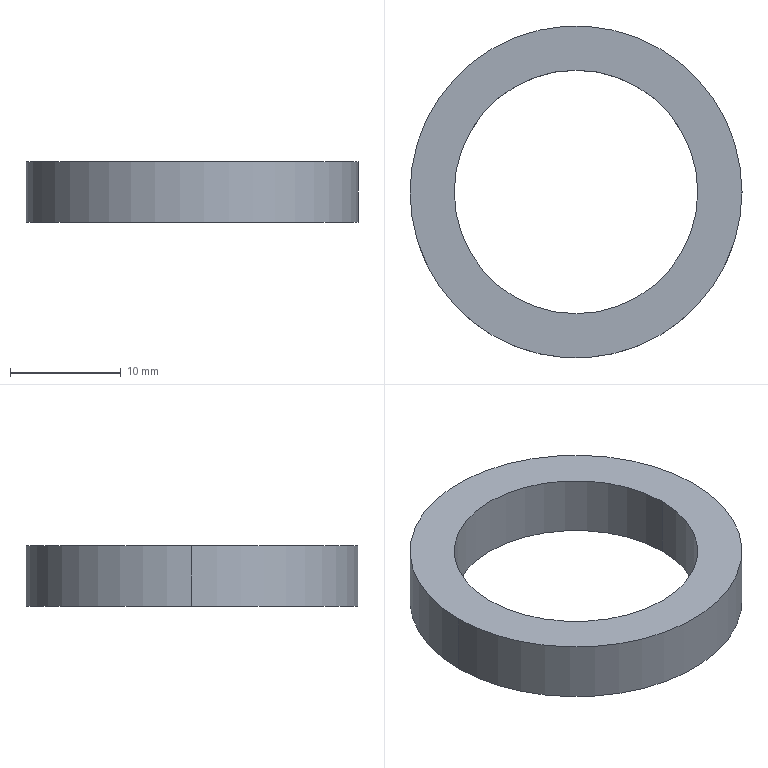Part | STEP file | CU AN TOAN 10.4-20 - 5.5 | 1 solid | 6 faces | box 30 x 30 x 5.5 mm | volume 1797 mm3 | cylinder 4 | plane 2 | commonest cylinder face diameters 22 x2 30 x2
STEP:
#1=CARTESIAN_POINT('',(0.,0.,0.));
#2=DIRECTION('',(0.,0.,1.));
#3=DIRECTION('',(1.,0.,0.));
#4=AXIS2_PLACEMENT_3D('',#1,#2,#3);
#5=CARTESIAN_POINT('',(15.,0.,0.));
#6=VERTEX_POINT('',#5);
#7=CARTESIAN_POINT('',(-15.,0.,0.));
#8=VERTEX_POINT('',#7);
#9=CARTESIAN_POINT('',(0.,0.,0.));
#10=DIRECTION('',(0.,0.,1.));
#11=DIRECTION('',(1.,0.,0.));
#12=AXIS2_PLACEMENT_3D('',#9,#10,#11);
#13=CIRCLE('',#12,15.);
#14=CARTESIAN_POINT('',(0.,0.,0.));
#15=DIRECTION('',(0.,0.,1.));
#16=DIRECTION('',(1.,0.,0.));
#17=AXIS2_PLACEMENT_3D('',#14,#15,#16);
#18=CYLINDRICAL_SURFACE('',#17,15.);
#19=CARTESIAN_POINT('',(0.,0.));
#20=DIRECTION('',(1.,0.));
#21=VECTOR('',#20,1.);
#22=LINE('',#19,#21);
#23=(GEOMETRIC_REPRESENTATION_CONTEXT(2)PARAMETRIC_REPRESENTATION_CONTEXT()REPRESENTATION_CONTEXT('',''));
#24=DEFINITIONAL_REPRESENTATION('',(#22),#23);
#25=PCURVE('',#18,#24);
#26=CARTESIAN_POINT('',(0.,0.,0.));
#27=DIRECTION('',(0.,0.,-1.));
#28=DIRECTION('',(-1.,0.,0.));
#29=AXIS2_PLACEMENT_3D('',#26,#27,#28);
#30=PLANE('',#29);
#31=CARTESIAN_POINT('',(-15.,0.));
#32=CARTESIAN_POINT('',(-15.,25.981));
#33=CARTESIAN_POINT('',(7.5,12.99));
#34=CARTESIAN_POINT('',(30.,0.));
#35=CARTESIAN_POINT('',(7.5,-12.99));
#36=CARTESIAN_POINT('',(-15.,-25.981));
#37=CARTESIAN_POINT('',(-15.,0.));
#38=(BOUNDED_CURVE()B_SPLINE_CURVE(2,(#31,#32,#33,#34,#35,#36,#37),.UNSPECIFIED.,.T.,.F.)B_SPLINE_CURVE_WITH_KNOTS((1,2,2,2,2,1),(-2.094,0.,2.094,4.189,6.283,8.378),.UNSPECIFIED.)CURVE()GEOMETRIC_REPRESENTATION_ITEM()RATIONAL_B_SPLINE_CURVE((1.,0.5,1.,0.5,1.,0.5,1.))REPRESENTATION_ITEM(''));
#39=(GEOMETRIC_REPRESENTATION_CONTEXT(2)PARAMETRIC_REPRESENTATION_CONTEXT()REPRESENTATION_CONTEXT('',''));
#40=DEFINITIONAL_REPRESENTATION('',(#38),#39);
#41=PCURVE('',#30,#40);
#42=SURFACE_CURVE('',#13,(#25,#41),.PCURVE_S1.);
#43=EDGE_CURVE('',#6,#8,#42,.T.);
#44=ORIENTED_EDGE('',*,*,#43,.T.);
#45=CARTESIAN_POINT('',(-15.,0.,5.5));
#46=VERTEX_POINT('',#45);
#47=CARTESIAN_POINT('',(-15.,0.,0.));
#48=DIRECTION('',(0.,0.,1.));
#49=VECTOR('',#48,1.);
#50=LINE('',#47,#49);
#51=CARTESIAN_POINT('',(3.142,0.));
#52=DIRECTION('',(0.,1.));
#53=VECTOR('',#52,1.);
#54=LINE('',#51,#53);
#55=(GEOMETRIC_REPRESENTATION_CONTEXT(2)PARAMETRIC_REPRESENTATION_CONTEXT()REPRESENTATION_CONTEXT('',''));
#56=DEFINITIONAL_REPRESENTATION('',(#54),#55);
#57=PCURVE('',#18,#56);
#58=CARTESIAN_POINT('',(0.,0.,0.));
#59=DIRECTION('',(0.,0.,1.));
#60=DIRECTION('',(1.,0.,0.));
#61=AXIS2_PLACEMENT_3D('',#58,#59,#60);
#62=CYLINDRICAL_SURFACE('',#61,15.);
#63=CARTESIAN_POINT('',(3.142,0.));
#64=DIRECTION('',(0.,1.));
#65=VECTOR('',#64,1.);
#66=LINE('',#63,#65);
#67=(GEOMETRIC_REPRESENTATION_CONTEXT(2)PARAMETRIC_REPRESENTATION_CONTEXT()REPRESENTATION_CONTEXT('',''));
#68=DEFINITIONAL_REPRESENTATION('',(#66),#67);
#69=PCURVE('',#62,#68);
#70=SURFACE_CURVE('',#50,(#57,#69),.PCURVE_S1.);
#71=EDGE_CURVE('',#8,#46,#70,.T.);
#72=ORIENTED_EDGE('',*,*,#71,.T.);
#73=CARTESIAN_POINT('',(15.,0.,5.5));
#74=VERTEX_POINT('',#73);
#75=CARTESIAN_POINT('',(0.,0.,5.5));
#76=DIRECTION('',(0.,0.,-1.));
#77=DIRECTION('',(1.,0.,0.));
#78=AXIS2_PLACEMENT_3D('',#75,#76,#77);
#79=CIRCLE('',#78,15.);
#80=CARTESIAN_POINT('',(6.283,5.5));
#81=DIRECTION('',(-1.,0.));
#82=VECTOR('',#81,1.);
#83=LINE('',#80,#82);
#84=(GEOMETRIC_REPRESENTATION_CONTEXT(2)PARAMETRIC_REPRESENTATION_CONTEXT()REPRESENTATION_CONTEXT('',''));
#85=DEFINITIONAL_REPRESENTATION('',(#83),#84);
#86=PCURVE('',#18,#85);
#87=CARTESIAN_POINT('',(0.,0.,5.5));
#88=DIRECTION('',(0.,0.,-1.));
#89=DIRECTION('',(-1.,0.,0.));
#90=AXIS2_PLACEMENT_3D('',#87,#88,#89);
#91=PLANE('',#90);
#92=CARTESIAN_POINT('',(0.,0.));
#93=DIRECTION('',(-1.,0.));
#94=AXIS2_PLACEMENT_2D('',#92,#93);
#95=CIRCLE('',#94,15.);
#96=(GEOMETRIC_REPRESENTATION_CONTEXT(2)PARAMETRIC_REPRESENTATION_CONTEXT()REPRESENTATION_CONTEXT('',''));
#97=DEFINITIONAL_REPRESENTATION('',(#95),#96);
#98=PCURVE('',#91,#97);
#99=SURFACE_CURVE('',#79,(#86,#98),.PCURVE_S1.);
#100=EDGE_CURVE('',#46,#74,#99,.T.);
#101=ORIENTED_EDGE('',*,*,#100,.T.);
#102=CARTESIAN_POINT('',(15.,0.,0.));
#103=DIRECTION('',(0.,0.,1.));
#104=VECTOR('',#103,1.);
#105=LINE('',#102,#104);
#106=CARTESIAN_POINT('',(0.,0.));
#107=DIRECTION('',(0.,1.));
#108=VECTOR('',#107,1.);
#109=LINE('',#106,#108);
#110=(GEOMETRIC_REPRESENTATION_CONTEXT(2)PARAMETRIC_REPRESENTATION_CONTEXT()REPRESENTATION_CONTEXT('',''));
#111=DEFINITIONAL_REPRESENTATION('',(#109),#110);
#112=PCURVE('',#18,#111);
#113=CARTESIAN_POINT('',(6.283,0.));
#114=DIRECTION('',(0.,1.));
#115=VECTOR('',#114,1.);
#116=LINE('',#113,#115);
#117=(GEOMETRIC_REPRESENTATION_CONTEXT(2)PARAMETRIC_REPRESENTATION_CONTEXT()REPRESENTATION_CONTEXT('',''));
#118=DEFINITIONAL_REPRESENTATION('',(#116),#117);
#119=PCURVE('',#62,#118);
#120=SURFACE_CURVE('',#105,(#112,#119),.PCURVE_S1.);
#121=EDGE_CURVE('',#6,#74,#120,.T.);
#122=ORIENTED_EDGE('',*,*,#121,.F.);
#123=EDGE_LOOP('',(#44,#72,#101,#122));
#124=FACE_BOUND('',#123,.T.);
#125=ADVANCED_FACE('',(#124),#18,.T.);
#126=CARTESIAN_POINT('',(11.,0.,0.));
#127=VERTEX_POINT('',#126);
#128=CARTESIAN_POINT('',(11.,0.,5.5));
#129=VERTEX_POINT('',#128);
#130=CARTESIAN_POINT('',(11.,0.,0.));
#131=DIRECTION('',(0.,0.,1.));
#132=VECTOR('',#131,1.);
#133=LINE('',#130,#132);
#134=CARTESIAN_POINT('',(0.,0.,0.));
#135=DIRECTION('',(0.,0.,1.));
#136=DIRECTION('',(1.,0.,0.));
#137=AXIS2_PLACEMENT_3D('',#134,#135,#136);
#138=CYLINDRICAL_SURFACE('',#137,11.);
#139=CARTESIAN_POINT('',(6.283,0.));
#140=DIRECTION('',(0.,1.));
#141=VECTOR('',#140,1.);
#142=LINE('',#139,#141);
#143=(GEOMETRIC_REPRESENTATION_CONTEXT(2)PARAMETRIC_REPRESENTATION_CONTEXT()REPRESENTATION_CONTEXT('',''));
#144=DEFINITIONAL_REPRESENTATION('',(#142),#143);
#145=PCURVE('',#138,#144);
#146=CARTESIAN_POINT('',(0.,0.,0.));
#147=DIRECTION('',(0.,0.,1.));
#148=DIRECTION('',(1.,0.,0.));
#149=AXIS2_PLACEMENT_3D('',#146,#147,#148);
#150=CYLINDRICAL_SURFACE('',#149,11.);
#151=CARTESIAN_POINT('',(0.,0.));
#152=DIRECTION('',(0.,1.));
#153=VECTOR('',#152,1.);
#154=LINE('',#151,#153);
#155=(GEOMETRIC_REPRESENTATION_CONTEXT(2)PARAMETRIC_REPRESENTATION_CONTEXT()REPRESENTATION_CONTEXT('',''));
#156=DEFINITIONAL_REPRESENTATION('',(#154),#155);
#157=PCURVE('',#150,#156);
#158=SURFACE_CURVE('',#133,(#145,#157),.PCURVE_S1.);
#159=EDGE_CURVE('',#127,#129,#158,.T.);
#160=ORIENTED_EDGE('',*,*,#159,.T.);
#161=CARTESIAN_POINT('',(-11.,0.,5.5));
#162=VERTEX_POINT('',#161);
#163=CARTESIAN_POINT('',(0.,0.,5.5));
#164=DIRECTION('',(0.,0.,1.));
#165=DIRECTION('',(1.,0.,0.));
#166=AXIS2_PLACEMENT_3D('',#163,#164,#165);
#167=CIRCLE('',#166,11.);
#168=CARTESIAN_POINT('',(0.,5.5));
#169=DIRECTION('',(1.,0.));
#170=VECTOR('',#169,1.);
#171=LINE('',#168,#170);
#172=(GEOMETRIC_REPRESENTATION_CONTEXT(2)PARAMETRIC_REPRESENTATION_CONTEXT()REPRESENTATION_CONTEXT('',''));
#173=DEFINITIONAL_REPRESENTATION('',(#171),#172);
#174=PCURVE('',#138,#173);
#175=CARTESIAN_POINT('',(-11.,0.));
#176=CARTESIAN_POINT('',(-11.,19.053));
#177=CARTESIAN_POINT('',(5.5,9.526));
#178=CARTESIAN_POINT('',(22.,0.));
#179=CARTESIAN_POINT('',(5.5,-9.526));
#180=CARTESIAN_POINT('',(-11.,-19.053));
#181=CARTESIAN_POINT('',(-11.,0.));
#182=(BOUNDED_CURVE()B_SPLINE_CURVE(2,(#175,#176,#177,#178,#179,#180,#181),.UNSPECIFIED.,.T.,.F.)B_SPLINE_CURVE_WITH_KNOTS((1,2,2,2,2,1),(-2.094,0.,2.094,4.189,6.283,8.378),.UNSPECIFIED.)CURVE()GEOMETRIC_REPRESENTATION_ITEM()RATIONAL_B_SPLINE_CURVE((1.,0.5,1.,0.5,1.,0.5,1.))REPRESENTATION_ITEM(''));
#183=(GEOMETRIC_REPRESENTATION_CONTEXT(2)PARAMETRIC_REPRESENTATION_CONTEXT()REPRESENTATION_CONTEXT('',''));
#184=DEFINITIONAL_REPRESENTATION('',(#182),#183);
#185=PCURVE('',#91,#184);
#186=SURFACE_CURVE('',#167,(#174,#185),.PCURVE_S1.);
#187=EDGE_CURVE('',#162,#129,#186,.T.);
#188=ORIENTED_EDGE('',*,*,#187,.F.);
#189=CARTESIAN_POINT('',(-11.,0.,0.));
#190=VERTEX_POINT('',#189);
#191=CARTESIAN_POINT('',(-11.,0.,0.));
#192=DIRECTION('',(0.,0.,1.));
#193=VECTOR('',#192,1.);
#194=LINE('',#191,#193);
#195=CARTESIAN_POINT('',(3.142,0.));
#196=DIRECTION('',(0.,1.));
#197=VECTOR('',#196,1.);
#198=LINE('',#195,#197);
#199=(GEOMETRIC_REPRESENTATION_CONTEXT(2)PARAMETRIC_REPRESENTATION_CONTEXT()REPRESENTATION_CONTEXT('',''));
#200=DEFINITIONAL_REPRESENTATION('',(#198),#199);
#201=PCURVE('',#138,#200);
#202=CARTESIAN_POINT('',(3.142,0.));
#203=DIRECTION('',(0.,1.));
#204=VECTOR('',#203,1.);
#205=LINE('',#202,#204);
#206=(GEOMETRIC_REPRESENTATION_CONTEXT(2)PARAMETRIC_REPRESENTATION_CONTEXT()REPRESENTATION_CONTEXT('',''));
#207=DEFINITIONAL_REPRESENTATION('',(#205),#206);
#208=PCURVE('',#150,#207);
#209=SURFACE_CURVE('',#194,(#201,#208),.PCURVE_S1.);
#210=EDGE_CURVE('',#190,#162,#209,.T.);
#211=ORIENTED_EDGE('',*,*,#210,.F.);
#212=CARTESIAN_POINT('',(0.,0.,0.));
#213=DIRECTION('',(0.,0.,1.));
#214=DIRECTION('',(1.,0.,0.));
#215=AXIS2_PLACEMENT_3D('',#212,#213,#214);
#216=CIRCLE('',#215,11.);
#217=CARTESIAN_POINT('',(0.,0.));
#218=DIRECTION('',(1.,0.));
#219=VECTOR('',#218,1.);
#220=LINE('',#217,#219);
#221=(GEOMETRIC_REPRESENTATION_CONTEXT(2)PARAMETRIC_REPRESENTATION_CONTEXT()REPRESENTATION_CONTEXT('',''));
#222=DEFINITIONAL_REPRESENTATION('',(#220),#221);
#223=PCURVE('',#138,#222);
#224=CARTESIAN_POINT('',(-11.,0.));
#225=CARTESIAN_POINT('',(-11.,19.053));
#226=CARTESIAN_POINT('',(5.5,9.526));
#227=CARTESIAN_POINT('',(22.,0.));
#228=CARTESIAN_POINT('',(5.5,-9.526));
#229=CARTESIAN_POINT('',(-11.,-19.053));
#230=CARTESIAN_POINT('',(-11.,0.));
#231=(BOUNDED_CURVE()B_SPLINE_CURVE(2,(#224,#225,#226,#227,#228,#229,#230),.UNSPECIFIED.,.T.,.F.)B_SPLINE_CURVE_WITH_KNOTS((1,2,2,2,2,1),(-2.094,0.,2.094,4.189,6.283,8.378),.UNSPECIFIED.)CURVE()GEOMETRIC_REPRESENTATION_ITEM()RATIONAL_B_SPLINE_CURVE((1.,0.5,1.,0.5,1.,0.5,1.))REPRESENTATION_ITEM(''));
#232=(GEOMETRIC_REPRESENTATION_CONTEXT(2)PARAMETRIC_REPRESENTATION_CONTEXT()REPRESENTATION_CONTEXT('',''));
#233=DEFINITIONAL_REPRESENTATION('',(#231),#232);
#234=PCURVE('',#30,#233);
#235=SURFACE_CURVE('',#216,(#223,#234),.PCURVE_S1.);
#236=EDGE_CURVE('',#190,#127,#235,.T.);
#237=ORIENTED_EDGE('',*,*,#236,.T.);
#238=EDGE_LOOP('',(#160,#188,#211,#237));
#239=FACE_BOUND('',#238,.F.);
#240=ADVANCED_FACE('',(#239),#138,.F.);
#241=ORIENTED_EDGE('',*,*,#71,.F.);
#242=CARTESIAN_POINT('',(0.,0.,0.));
#243=DIRECTION('',(0.,0.,1.));
#244=DIRECTION('',(1.,0.,0.));
#245=AXIS2_PLACEMENT_3D('',#242,#243,#244);
#246=CIRCLE('',#245,15.);
#247=CARTESIAN_POINT('',(0.,0.));
#248=DIRECTION('',(1.,0.));
#249=VECTOR('',#248,1.);
#250=LINE('',#247,#249);
#251=(GEOMETRIC_REPRESENTATION_CONTEXT(2)PARAMETRIC_REPRESENTATION_CONTEXT()REPRESENTATION_CONTEXT('',''));
#252=DEFINITIONAL_REPRESENTATION('',(#250),#251);
#253=PCURVE('',#62,#252);
#254=CARTESIAN_POINT('',(-15.,0.));
#255=CARTESIAN_POINT('',(-15.,25.981));
#256=CARTESIAN_POINT('',(7.5,12.99));
#257=CARTESIAN_POINT('',(30.,0.));
#258=CARTESIAN_POINT('',(7.5,-12.99));
#259=CARTESIAN_POINT('',(-15.,-25.981));
#260=CARTESIAN_POINT('',(-15.,0.));
#261=(BOUNDED_CURVE()B_SPLINE_CURVE(2,(#254,#255,#256,#257,#258,#259,#260),.UNSPECIFIED.,.T.,.F.)B_SPLINE_CURVE_WITH_KNOTS((1,2,2,2,2,1),(-2.094,0.,2.094,4.189,6.283,8.378),.UNSPECIFIED.)CURVE()GEOMETRIC_REPRESENTATION_ITEM()RATIONAL_B_SPLINE_CURVE((1.,0.5,1.,0.5,1.,0.5,1.))REPRESENTATION_ITEM(''));
#262=(GEOMETRIC_REPRESENTATION_CONTEXT(2)PARAMETRIC_REPRESENTATION_CONTEXT()REPRESENTATION_CONTEXT('',''));
#263=DEFINITIONAL_REPRESENTATION('',(#261),#262);
#264=PCURVE('',#30,#263);
#265=SURFACE_CURVE('',#246,(#253,#264),.PCURVE_S1.);
#266=EDGE_CURVE('',#8,#6,#265,.T.);
#267=ORIENTED_EDGE('',*,*,#266,.T.);
#268=ORIENTED_EDGE('',*,*,#121,.T.);
#269=CARTESIAN_POINT('',(0.,0.,5.5));
#270=DIRECTION('',(0.,0.,-1.));
#271=DIRECTION('',(1.,0.,0.));
#272=AXIS2_PLACEMENT_3D('',#269,#270,#271);
#273=CIRCLE('',#272,15.);
#274=CARTESIAN_POINT('',(6.283,5.5));
#275=DIRECTION('',(-1.,0.));
#276=VECTOR('',#275,1.);
#277=LINE('',#274,#276);
#278=(GEOMETRIC_REPRESENTATION_CONTEXT(2)PARAMETRIC_REPRESENTATION_CONTEXT()REPRESENTATION_CONTEXT('',''));
#279=DEFINITIONAL_REPRESENTATION('',(#277),#278);
#280=PCURVE('',#62,#279);
#281=CARTESIAN_POINT('',(0.,0.));
#282=DIRECTION('',(-1.,0.));
#283=AXIS2_PLACEMENT_2D('',#281,#282);
#284=CIRCLE('',#283,15.);
#285=(GEOMETRIC_REPRESENTATION_CONTEXT(2)PARAMETRIC_REPRESENTATION_CONTEXT()REPRESENTATION_CONTEXT('',''));
#286=DEFINITIONAL_REPRESENTATION('',(#284),#285);
#287=PCURVE('',#91,#286);
#288=SURFACE_CURVE('',#273,(#280,#287),.PCURVE_S1.);
#289=EDGE_CURVE('',#74,#46,#288,.T.);
#290=ORIENTED_EDGE('',*,*,#289,.T.);
#291=EDGE_LOOP('',(#241,#267,#268,#290));
#292=FACE_BOUND('',#291,.T.);
#293=ADVANCED_FACE('',(#292),#62,.T.);
#294=CARTESIAN_POINT('',(0.,0.,0.));
#295=DIRECTION('',(0.,0.,1.));
#296=DIRECTION('',(1.,0.,0.));
#297=AXIS2_PLACEMENT_3D('',#294,#295,#296);
#298=CIRCLE('',#297,11.);
#299=CARTESIAN_POINT('',(-11.,0.));
#300=CARTESIAN_POINT('',(-11.,19.053));
#301=CARTESIAN_POINT('',(5.5,9.526));
#302=CARTESIAN_POINT('',(22.,0.));
#303=CARTESIAN_POINT('',(5.5,-9.526));
#304=CARTESIAN_POINT('',(-11.,-19.053));
#305=CARTESIAN_POINT('',(-11.,0.));
#306=(BOUNDED_CURVE()B_SPLINE_CURVE(2,(#299,#300,#301,#302,#303,#304,#305),.UNSPECIFIED.,.T.,.F.)B_SPLINE_CURVE_WITH_KNOTS((1,2,2,2,2,1),(-2.094,0.,2.094,4.189,6.283,8.378),.UNSPECIFIED.)CURVE()GEOMETRIC_REPRESENTATION_ITEM()RATIONAL_B_SPLINE_CURVE((1.,0.5,1.,0.5,1.,0.5,1.))REPRESENTATION_ITEM(''));
#307=(GEOMETRIC_REPRESENTATION_CONTEXT(2)PARAMETRIC_REPRESENTATION_CONTEXT()REPRESENTATION_CONTEXT('',''));
#308=DEFINITIONAL_REPRESENTATION('',(#306),#307);
#309=PCURVE('',#30,#308);
#310=CARTESIAN_POINT('',(0.,0.));
#311=DIRECTION('',(1.,0.));
#312=VECTOR('',#311,1.);
#313=LINE('',#310,#312);
#314=(GEOMETRIC_REPRESENTATION_CONTEXT(2)PARAMETRIC_REPRESENTATION_CONTEXT()REPRESENTATION_CONTEXT('',''));
#315=DEFINITIONAL_REPRESENTATION('',(#313),#314);
#316=PCURVE('',#150,#315);
#317=SURFACE_CURVE('',#298,(#309,#316),.PCURVE_S1.);
#318=EDGE_CURVE('',#127,#190,#317,.T.);
#319=ORIENTED_EDGE('',*,*,#318,.T.);
#320=ORIENTED_EDGE('',*,*,#236,.T.);
#321=EDGE_LOOP('',(#319,#320));
#322=FACE_BOUND('',#321,.T.);
#323=ORIENTED_EDGE('',*,*,#43,.F.);
#324=ORIENTED_EDGE('',*,*,#266,.F.);
#325=EDGE_LOOP('',(#323,#324));
#326=FACE_BOUND('',#325,.T.);
#327=ADVANCED_FACE('',(#322,#326),#30,.T.);
#328=CARTESIAN_POINT('',(0.,0.,5.5));
#329=DIRECTION('',(0.,0.,1.));
#330=DIRECTION('',(1.,0.,0.));
#331=AXIS2_PLACEMENT_3D('',#328,#329,#330);
#332=CIRCLE('',#331,11.);
#333=CARTESIAN_POINT('',(-11.,0.));
#334=CARTESIAN_POINT('',(-11.,19.053));
#335=CARTESIAN_POINT('',(5.5,9.526));
#336=CARTESIAN_POINT('',(22.,0.));
#337=CARTESIAN_POINT('',(5.5,-9.526));
#338=CARTESIAN_POINT('',(-11.,-19.053));
#339=CARTESIAN_POINT('',(-11.,0.));
#340=(BOUNDED_CURVE()B_SPLINE_CURVE(2,(#333,#334,#335,#336,#337,#338,#339),.UNSPECIFIED.,.T.,.F.)B_SPLINE_CURVE_WITH_KNOTS((1,2,2,2,2,1),(-2.094,0.,2.094,4.189,6.283,8.378),.UNSPECIFIED.)CURVE()GEOMETRIC_REPRESENTATION_ITEM()RATIONAL_B_SPLINE_CURVE((1.,0.5,1.,0.5,1.,0.5,1.))REPRESENTATION_ITEM(''));
#341=(GEOMETRIC_REPRESENTATION_CONTEXT(2)PARAMETRIC_REPRESENTATION_CONTEXT()REPRESENTATION_CONTEXT('',''));
#342=DEFINITIONAL_REPRESENTATION('',(#340),#341);
#343=PCURVE('',#91,#342);
#344=CARTESIAN_POINT('',(0.,5.5));
#345=DIRECTION('',(1.,0.));
#346=VECTOR('',#345,1.);
#347=LINE('',#344,#346);
#348=(GEOMETRIC_REPRESENTATION_CONTEXT(2)PARAMETRIC_REPRESENTATION_CONTEXT()REPRESENTATION_CONTEXT('',''));
#349=DEFINITIONAL_REPRESENTATION('',(#347),#348);
#350=PCURVE('',#150,#349);
#351=SURFACE_CURVE('',#332,(#343,#350),.PCURVE_S1.);
#352=EDGE_CURVE('',#129,#162,#351,.T.);
#353=ORIENTED_EDGE('',*,*,#352,.F.);
#354=ORIENTED_EDGE('',*,*,#187,.F.);
#355=EDGE_LOOP('',(#353,#354));
#356=FACE_BOUND('',#355,.T.);
#357=ORIENTED_EDGE('',*,*,#289,.F.);
#358=ORIENTED_EDGE('',*,*,#100,.F.);
#359=EDGE_LOOP('',(#357,#358));
#360=FACE_BOUND('',#359,.T.);
#361=ADVANCED_FACE('',(#356,#360),#91,.F.);
#362=ORIENTED_EDGE('',*,*,#352,.F.);
#363=ORIENTED_EDGE('',*,*,#159,.F.);
#364=ORIENTED_EDGE('',*,*,#318,.T.);
#365=ORIENTED_EDGE('',*,*,#210,.T.);
#366=EDGE_LOOP('',(#362,#363,#364,#365));
#367=FACE_BOUND('',#366,.F.);
#368=ADVANCED_FACE('',(#367),#150,.F.);
#369=CLOSED_SHELL('',(#125,#240,#293,#327,#361,#368));
#370=MANIFOLD_SOLID_BREP('',#369);
#371=(LENGTH_UNIT()NAMED_UNIT(*)SI_UNIT(.MILLI.,.METRE.));
#372=UNCERTAINTY_MEASURE_WITH_UNIT(LENGTH_MEASURE(0.0000001),#371,'','');
#373=(NAMED_UNIT(*)PLANE_ANGLE_UNIT()SI_UNIT($,.RADIAN.));
#374=(NAMED_UNIT(*)SI_UNIT($,.STERADIAN.)SOLID_ANGLE_UNIT());
#375=(GEOMETRIC_REPRESENTATION_CONTEXT(3)GLOBAL_UNCERTAINTY_ASSIGNED_CONTEXT((#372))GLOBAL_UNIT_ASSIGNED_CONTEXT((#371,#373,#374))REPRESENTATION_CONTEXT('',''));
#376=ADVANCED_BREP_SHAPE_REPRESENTATION('',(#4,#370),#375);